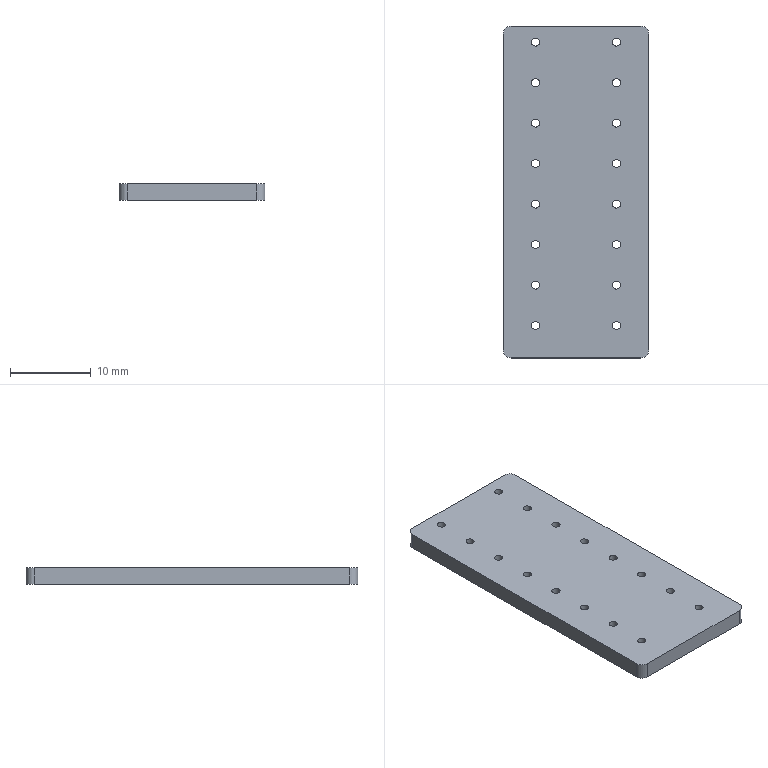Part | NX | features EXTRACT_BODY 7, DATUM_CSYS 3, EXTRUDE 2, SKETCH 2, Pattern Geometry 1, SUBTRACT 1 | 1 solid | 26 faces | box 18 x 41 x 2 mm | volume 1449 mm3 | cylinder 20 | plane 6 | commonest cylinder face diameters 1 x16 2 x4
STEP:
#1=CARTESIAN_POINT('',(-4.5,3.5,0.));
#2=VERTEX_POINT('',#1);
#3=CARTESIAN_POINT('',(-5.,3.5,0.));
#4=DIRECTION('',(0.,0.,1.));
#5=DIRECTION('',(1.,0.,0.));
#6=AXIS2_PLACEMENT_3D('',#3,#4,#5);
#7=CIRCLE('',#6,0.5);
#8=EDGE_CURVE('',#2,#2,#7,.T.);
#9=ORIENTED_EDGE('',*,*,#8,.T.);
#10=EDGE_LOOP('',(#9));
#11=FACE_BOUND('',#10,.T.);
#12=CARTESIAN_POINT('',(-4.5,-1.5,0.));
#13=VERTEX_POINT('',#12);
#14=CARTESIAN_POINT('',(-5.,-1.5,0.));
#15=DIRECTION('',(0.,0.,1.));
#16=DIRECTION('',(1.,0.,0.));
#17=AXIS2_PLACEMENT_3D('',#14,#15,#16);
#18=CIRCLE('',#17,0.5);
#19=EDGE_CURVE('',#13,#13,#18,.T.);
#20=ORIENTED_EDGE('',*,*,#19,.T.);
#21=EDGE_LOOP('',(#20));
#22=FACE_BOUND('',#21,.T.);
#23=CARTESIAN_POINT('',(-4.5,13.5,0.));
#24=VERTEX_POINT('',#23);
#25=CARTESIAN_POINT('',(-5.,13.5,0.));
#26=DIRECTION('',(0.,0.,1.));
#27=DIRECTION('',(1.,0.,0.));
#28=AXIS2_PLACEMENT_3D('',#25,#26,#27);
#29=CIRCLE('',#28,0.5);
#30=EDGE_CURVE('',#24,#24,#29,.T.);
#31=ORIENTED_EDGE('',*,*,#30,.T.);
#32=EDGE_LOOP('',(#31));
#33=FACE_BOUND('',#32,.T.);
#34=CARTESIAN_POINT('',(-4.5,8.5,0.));
#35=VERTEX_POINT('',#34);
#36=CARTESIAN_POINT('',(-5.,8.5,0.));
#37=DIRECTION('',(0.,0.,1.));
#38=DIRECTION('',(1.,0.,0.));
#39=AXIS2_PLACEMENT_3D('',#36,#37,#38);
#40=CIRCLE('',#39,0.5);
#41=EDGE_CURVE('',#35,#35,#40,.T.);
#42=ORIENTED_EDGE('',*,*,#41,.T.);
#43=EDGE_LOOP('',(#42));
#44=FACE_BOUND('',#43,.T.);
#45=CARTESIAN_POINT('',(-4.5,-16.5,0.));
#46=VERTEX_POINT('',#45);
#47=CARTESIAN_POINT('',(-5.,-16.5,0.));
#48=DIRECTION('',(0.,0.,1.));
#49=DIRECTION('',(1.,0.,0.));
#50=AXIS2_PLACEMENT_3D('',#47,#48,#49);
#51=CIRCLE('',#50,0.5);
#52=EDGE_CURVE('',#46,#46,#51,.T.);
#53=ORIENTED_EDGE('',*,*,#52,.T.);
#54=EDGE_LOOP('',(#53));
#55=FACE_BOUND('',#54,.T.);
#56=CARTESIAN_POINT('',(-4.5,-6.5,0.));
#57=VERTEX_POINT('',#56);
#58=CARTESIAN_POINT('',(-5.,-6.5,0.));
#59=DIRECTION('',(0.,0.,1.));
#60=DIRECTION('',(1.,0.,0.));
#61=AXIS2_PLACEMENT_3D('',#58,#59,#60);
#62=CIRCLE('',#61,0.5);
#63=EDGE_CURVE('',#57,#57,#62,.T.);
#64=ORIENTED_EDGE('',*,*,#63,.T.);
#65=EDGE_LOOP('',(#64));
#66=FACE_BOUND('',#65,.T.);
#67=CARTESIAN_POINT('',(-4.5,-11.5,0.));
#68=VERTEX_POINT('',#67);
#69=CARTESIAN_POINT('',(-5.,-11.5,0.));
#70=DIRECTION('',(0.,0.,1.));
#71=DIRECTION('',(1.,0.,0.));
#72=AXIS2_PLACEMENT_3D('',#69,#70,#71);
#73=CIRCLE('',#72,0.5);
#74=EDGE_CURVE('',#68,#68,#73,.T.);
#75=ORIENTED_EDGE('',*,*,#74,.T.);
#76=EDGE_LOOP('',(#75));
#77=FACE_BOUND('',#76,.T.);
#78=CARTESIAN_POINT('',(-4.5,18.5,0.));
#79=VERTEX_POINT('',#78);
#80=CARTESIAN_POINT('',(-5.,18.5,0.));
#81=DIRECTION('',(0.,0.,1.));
#82=DIRECTION('',(1.,0.,0.));
#83=AXIS2_PLACEMENT_3D('',#80,#81,#82);
#84=CIRCLE('',#83,0.5);
#85=EDGE_CURVE('',#79,#79,#84,.T.);
#86=ORIENTED_EDGE('',*,*,#85,.T.);
#87=EDGE_LOOP('',(#86));
#88=FACE_BOUND('',#87,.T.);
#89=CARTESIAN_POINT('',(-9.,19.5,0.));
#90=VERTEX_POINT('',#89);
#91=CARTESIAN_POINT('',(-9.,-19.5,0.));
#92=VERTEX_POINT('',#91);
#93=CARTESIAN_POINT('',(-9.,19.5,0.));
#94=DIRECTION('',(0.,-1.,0.));
#95=VECTOR('',#94,1000.);
#96=LINE('',#93,#95);
#97=EDGE_CURVE('',#90,#92,#96,.T.);
#98=ORIENTED_EDGE('',*,*,#97,.F.);
#99=CARTESIAN_POINT('',(-8.,20.5,0.));
#100=VERTEX_POINT('',#99);
#101=CARTESIAN_POINT('',(-8.,19.5,0.));
#102=DIRECTION('',(0.,0.,1.));
#103=DIRECTION('',(1.,0.,0.));
#104=AXIS2_PLACEMENT_3D('',#101,#102,#103);
#105=CIRCLE('',#104,1.);
#106=EDGE_CURVE('',#100,#90,#105,.T.);
#107=ORIENTED_EDGE('',*,*,#106,.F.);
#108=CARTESIAN_POINT('',(8.,20.5,0.));
#109=VERTEX_POINT('',#108);
#110=CARTESIAN_POINT('',(8.,20.5,0.));
#111=DIRECTION('',(-1.,0.,0.));
#112=VECTOR('',#111,1000.);
#113=LINE('',#110,#112);
#114=EDGE_CURVE('',#109,#100,#113,.T.);
#115=ORIENTED_EDGE('',*,*,#114,.F.);
#116=CARTESIAN_POINT('',(9.,19.5,0.));
#117=VERTEX_POINT('',#116);
#118=CARTESIAN_POINT('',(8.,19.5,0.));
#119=DIRECTION('',(0.,0.,1.));
#120=DIRECTION('',(1.,0.,0.));
#121=AXIS2_PLACEMENT_3D('',#118,#119,#120);
#122=CIRCLE('',#121,1.);
#123=EDGE_CURVE('',#117,#109,#122,.T.);
#124=ORIENTED_EDGE('',*,*,#123,.F.);
#125=CARTESIAN_POINT('',(9.,-19.5,0.));
#126=VERTEX_POINT('',#125);
#127=CARTESIAN_POINT('',(9.,-19.5,0.));
#128=DIRECTION('',(0.,1.,0.));
#129=VECTOR('',#128,1000.);
#130=LINE('',#127,#129);
#131=EDGE_CURVE('',#126,#117,#130,.T.);
#132=ORIENTED_EDGE('',*,*,#131,.F.);
#133=CARTESIAN_POINT('',(8.,-20.5,0.));
#134=VERTEX_POINT('',#133);
#135=CARTESIAN_POINT('',(8.,-19.5,0.));
#136=DIRECTION('',(0.,0.,1.));
#137=DIRECTION('',(1.,0.,0.));
#138=AXIS2_PLACEMENT_3D('',#135,#136,#137);
#139=CIRCLE('',#138,1.);
#140=EDGE_CURVE('',#134,#126,#139,.T.);
#141=ORIENTED_EDGE('',*,*,#140,.F.);
#142=CARTESIAN_POINT('',(-8.,-20.5,0.));
#143=VERTEX_POINT('',#142);
#144=CARTESIAN_POINT('',(-8.,-20.5,0.));
#145=DIRECTION('',(1.,0.,0.));
#146=VECTOR('',#145,1000.);
#147=LINE('',#144,#146);
#148=EDGE_CURVE('',#143,#134,#147,.T.);
#149=ORIENTED_EDGE('',*,*,#148,.F.);
#150=CARTESIAN_POINT('',(-8.,-19.5,0.));
#151=DIRECTION('',(0.,0.,1.));
#152=DIRECTION('',(1.,0.,0.));
#153=AXIS2_PLACEMENT_3D('',#150,#151,#152);
#154=CIRCLE('',#153,1.);
#155=EDGE_CURVE('',#92,#143,#154,.T.);
#156=ORIENTED_EDGE('',*,*,#155,.F.);
#157=EDGE_LOOP('',(#98,#107,#115,#124,#132,#141,#149,#156));
#158=FACE_BOUND('',#157,.T.);
#159=CARTESIAN_POINT('',(5.5,-6.5,0.));
#160=VERTEX_POINT('',#159);
#161=CARTESIAN_POINT('',(5.,-6.5,0.));
#162=DIRECTION('',(0.,0.,1.));
#163=DIRECTION('',(1.,0.,0.));
#164=AXIS2_PLACEMENT_3D('',#161,#162,#163);
#165=CIRCLE('',#164,0.5);
#166=EDGE_CURVE('',#160,#160,#165,.F.);
#167=ORIENTED_EDGE('',*,*,#166,.F.);
#168=EDGE_LOOP('',(#167));
#169=FACE_BOUND('',#168,.T.);
#170=CARTESIAN_POINT('',(5.5,-1.5,0.));
#171=VERTEX_POINT('',#170);
#172=CARTESIAN_POINT('',(5.,-1.5,0.));
#173=DIRECTION('',(0.,0.,1.));
#174=DIRECTION('',(1.,0.,0.));
#175=AXIS2_PLACEMENT_3D('',#172,#173,#174);
#176=CIRCLE('',#175,0.5);
#177=EDGE_CURVE('',#171,#171,#176,.F.);
#178=ORIENTED_EDGE('',*,*,#177,.F.);
#179=EDGE_LOOP('',(#178));
#180=FACE_BOUND('',#179,.T.);
#181=CARTESIAN_POINT('',(5.5,-16.5,0.));
#182=VERTEX_POINT('',#181);
#183=CARTESIAN_POINT('',(5.,-16.5,0.));
#184=DIRECTION('',(0.,0.,1.));
#185=DIRECTION('',(1.,0.,0.));
#186=AXIS2_PLACEMENT_3D('',#183,#184,#185);
#187=CIRCLE('',#186,0.5);
#188=EDGE_CURVE('',#182,#182,#187,.F.);
#189=ORIENTED_EDGE('',*,*,#188,.F.);
#190=EDGE_LOOP('',(#189));
#191=FACE_BOUND('',#190,.T.);
#192=CARTESIAN_POINT('',(5.5,-11.5,0.));
#193=VERTEX_POINT('',#192);
#194=CARTESIAN_POINT('',(5.,-11.5,0.));
#195=DIRECTION('',(0.,0.,1.));
#196=DIRECTION('',(1.,0.,0.));
#197=AXIS2_PLACEMENT_3D('',#194,#195,#196);
#198=CIRCLE('',#197,0.5);
#199=EDGE_CURVE('',#193,#193,#198,.F.);
#200=ORIENTED_EDGE('',*,*,#199,.F.);
#201=EDGE_LOOP('',(#200));
#202=FACE_BOUND('',#201,.T.);
#203=CARTESIAN_POINT('',(5.5,13.5,0.));
#204=VERTEX_POINT('',#203);
#205=CARTESIAN_POINT('',(5.,13.5,0.));
#206=DIRECTION('',(0.,0.,1.));
#207=DIRECTION('',(1.,0.,0.));
#208=AXIS2_PLACEMENT_3D('',#205,#206,#207);
#209=CIRCLE('',#208,0.5);
#210=EDGE_CURVE('',#204,#204,#209,.F.);
#211=ORIENTED_EDGE('',*,*,#210,.F.);
#212=EDGE_LOOP('',(#211));
#213=FACE_BOUND('',#212,.T.);
#214=CARTESIAN_POINT('',(5.5,18.5,0.));
#215=VERTEX_POINT('',#214);
#216=CARTESIAN_POINT('',(5.,18.5,0.));
#217=DIRECTION('',(0.,0.,1.));
#218=DIRECTION('',(1.,0.,0.));
#219=AXIS2_PLACEMENT_3D('',#216,#217,#218);
#220=CIRCLE('',#219,0.5);
#221=EDGE_CURVE('',#215,#215,#220,.F.);
#222=ORIENTED_EDGE('',*,*,#221,.F.);
#223=EDGE_LOOP('',(#222));
#224=FACE_BOUND('',#223,.T.);
#225=CARTESIAN_POINT('',(5.5,3.5,0.));
#226=VERTEX_POINT('',#225);
#227=CARTESIAN_POINT('',(5.,3.5,0.));
#228=DIRECTION('',(0.,0.,1.));
#229=DIRECTION('',(1.,0.,0.));
#230=AXIS2_PLACEMENT_3D('',#227,#228,#229);
#231=CIRCLE('',#230,0.5);
#232=EDGE_CURVE('',#226,#226,#231,.F.);
#233=ORIENTED_EDGE('',*,*,#232,.F.);
#234=EDGE_LOOP('',(#233));
#235=FACE_BOUND('',#234,.T.);
#236=CARTESIAN_POINT('',(5.5,8.5,0.));
#237=VERTEX_POINT('',#236);
#238=CARTESIAN_POINT('',(5.,8.5,0.));
#239=DIRECTION('',(0.,0.,1.));
#240=DIRECTION('',(1.,0.,0.));
#241=AXIS2_PLACEMENT_3D('',#238,#239,#240);
#242=CIRCLE('',#241,0.5);
#243=EDGE_CURVE('',#237,#237,#242,.F.);
#244=ORIENTED_EDGE('',*,*,#243,.F.);
#245=EDGE_LOOP('',(#244));
#246=FACE_BOUND('',#245,.T.);
#247=CARTESIAN_POINT('',(-8.,-19.5,0.));
#248=DIRECTION('',(0.,0.,1.));
#249=DIRECTION('',(1.,0.,0.));
#250=AXIS2_PLACEMENT_3D('',#247,#248,#249);
#251=PLANE('',#250);
#252=ADVANCED_FACE('',(#11,#22,#33,#44,#55,#66,#77,#88,#158,#169,#180,#191,#202,#213,#224,#235,#246),#251,.F.);
#253=CARTESIAN_POINT('',(5.5,3.5,2.));
#254=VERTEX_POINT('',#253);
#255=CARTESIAN_POINT('',(5.,3.5,2.));
#256=DIRECTION('',(0.,0.,1.));
#257=DIRECTION('',(1.,0.,0.));
#258=AXIS2_PLACEMENT_3D('',#255,#256,#257);
#259=CIRCLE('',#258,0.5);
#260=EDGE_CURVE('',#254,#254,#259,.F.);
#261=ORIENTED_EDGE('',*,*,#260,.T.);
#262=EDGE_LOOP('',(#261));
#263=FACE_BOUND('',#262,.T.);
#264=CARTESIAN_POINT('',(-4.5,-1.5,2.));
#265=VERTEX_POINT('',#264);
#266=CARTESIAN_POINT('',(-5.,-1.5,2.));
#267=DIRECTION('',(0.,0.,1.));
#268=DIRECTION('',(1.,0.,0.));
#269=AXIS2_PLACEMENT_3D('',#266,#267,#268);
#270=CIRCLE('',#269,0.5);
#271=EDGE_CURVE('',#265,#265,#270,.T.);
#272=ORIENTED_EDGE('',*,*,#271,.F.);
#273=EDGE_LOOP('',(#272));
#274=FACE_BOUND('',#273,.T.);
#275=CARTESIAN_POINT('',(5.5,13.5,2.));
#276=VERTEX_POINT('',#275);
#277=CARTESIAN_POINT('',(5.,13.5,2.));
#278=DIRECTION('',(0.,0.,1.));
#279=DIRECTION('',(1.,0.,0.));
#280=AXIS2_PLACEMENT_3D('',#277,#278,#279);
#281=CIRCLE('',#280,0.5);
#282=EDGE_CURVE('',#276,#276,#281,.F.);
#283=ORIENTED_EDGE('',*,*,#282,.T.);
#284=EDGE_LOOP('',(#283));
#285=FACE_BOUND('',#284,.T.);
#286=CARTESIAN_POINT('',(-4.5,8.5,2.));
#287=VERTEX_POINT('',#286);
#288=CARTESIAN_POINT('',(-5.,8.5,2.));
#289=DIRECTION('',(0.,0.,1.));
#290=DIRECTION('',(1.,0.,0.));
#291=AXIS2_PLACEMENT_3D('',#288,#289,#290);
#292=CIRCLE('',#291,0.5);
#293=EDGE_CURVE('',#287,#287,#292,.T.);
#294=ORIENTED_EDGE('',*,*,#293,.F.);
#295=EDGE_LOOP('',(#294));
#296=FACE_BOUND('',#295,.T.);
#297=CARTESIAN_POINT('',(5.5,-16.5,2.));
#298=VERTEX_POINT('',#297);
#299=CARTESIAN_POINT('',(5.,-16.5,2.));
#300=DIRECTION('',(0.,0.,1.));
#301=DIRECTION('',(1.,0.,0.));
#302=AXIS2_PLACEMENT_3D('',#299,#300,#301);
#303=CIRCLE('',#302,0.5);
#304=EDGE_CURVE('',#298,#298,#303,.F.);
#305=ORIENTED_EDGE('',*,*,#304,.T.);
#306=EDGE_LOOP('',(#305));
#307=FACE_BOUND('',#306,.T.);
#308=CARTESIAN_POINT('',(5.5,-6.5,2.));
#309=VERTEX_POINT('',#308);
#310=CARTESIAN_POINT('',(5.,-6.5,2.));
#311=DIRECTION('',(0.,0.,1.));
#312=DIRECTION('',(1.,0.,0.));
#313=AXIS2_PLACEMENT_3D('',#310,#311,#312);
#314=CIRCLE('',#313,0.5);
#315=EDGE_CURVE('',#309,#309,#314,.F.);
#316=ORIENTED_EDGE('',*,*,#315,.T.);
#317=EDGE_LOOP('',(#316));
#318=FACE_BOUND('',#317,.T.);
#319=CARTESIAN_POINT('',(-4.5,-11.5,2.));
#320=VERTEX_POINT('',#319);
#321=CARTESIAN_POINT('',(-5.,-11.5,2.));
#322=DIRECTION('',(0.,0.,1.));
#323=DIRECTION('',(1.,0.,0.));
#324=AXIS2_PLACEMENT_3D('',#321,#322,#323);
#325=CIRCLE('',#324,0.5);
#326=EDGE_CURVE('',#320,#320,#325,.T.);
#327=ORIENTED_EDGE('',*,*,#326,.F.);
#328=EDGE_LOOP('',(#327));
#329=FACE_BOUND('',#328,.T.);
#330=CARTESIAN_POINT('',(-4.5,18.5,2.));
#331=VERTEX_POINT('',#330);
#332=CARTESIAN_POINT('',(-5.,18.5,2.));
#333=DIRECTION('',(0.,0.,1.));
#334=DIRECTION('',(1.,0.,0.));
#335=AXIS2_PLACEMENT_3D('',#332,#333,#334);
#336=CIRCLE('',#335,0.5);
#337=EDGE_CURVE('',#331,#331,#336,.T.);
#338=ORIENTED_EDGE('',*,*,#337,.F.);
#339=EDGE_LOOP('',(#338));
#340=FACE_BOUND('',#339,.T.);
#341=CARTESIAN_POINT('',(-9.,19.5,2.));
#342=VERTEX_POINT('',#341);
#343=CARTESIAN_POINT('',(-9.,-19.5,2.));
#344=VERTEX_POINT('',#343);
#345=CARTESIAN_POINT('',(-9.,19.5,2.));
#346=DIRECTION('',(0.,-1.,0.));
#347=VECTOR('',#346,1000.);
#348=LINE('',#345,#347);
#349=EDGE_CURVE('',#342,#344,#348,.T.);
#350=ORIENTED_EDGE('',*,*,#349,.T.);
#351=CARTESIAN_POINT('',(-8.,-20.5,2.));
#352=VERTEX_POINT('',#351);
#353=CARTESIAN_POINT('',(-8.,-19.5,2.));
#354=DIRECTION('',(0.,0.,1.));
#355=DIRECTION('',(1.,0.,0.));
#356=AXIS2_PLACEMENT_3D('',#353,#354,#355);
#357=CIRCLE('',#356,1.);
#358=EDGE_CURVE('',#344,#352,#357,.T.);
#359=ORIENTED_EDGE('',*,*,#358,.T.);
#360=CARTESIAN_POINT('',(8.,-20.5,2.));
#361=VERTEX_POINT('',#360);
#362=CARTESIAN_POINT('',(-8.,-20.5,2.));
#363=DIRECTION('',(1.,0.,0.));
#364=VECTOR('',#363,1000.);
#365=LINE('',#362,#364);
#366=EDGE_CURVE('',#352,#361,#365,.T.);
#367=ORIENTED_EDGE('',*,*,#366,.T.);
#368=CARTESIAN_POINT('',(9.,-19.5,2.));
#369=VERTEX_POINT('',#368);
#370=CARTESIAN_POINT('',(8.,-19.5,2.));
#371=DIRECTION('',(0.,0.,1.));
#372=DIRECTION('',(1.,0.,0.));
#373=AXIS2_PLACEMENT_3D('',#370,#371,#372);
#374=CIRCLE('',#373,1.);
#375=EDGE_CURVE('',#361,#369,#374,.T.);
#376=ORIENTED_EDGE('',*,*,#375,.T.);
#377=CARTESIAN_POINT('',(9.,19.5,2.));
#378=VERTEX_POINT('',#377);
#379=CARTESIAN_POINT('',(9.,-19.5,2.));
#380=DIRECTION('',(0.,1.,0.));
#381=VECTOR('',#380,1000.);
#382=LINE('',#379,#381);
#383=EDGE_CURVE('',#369,#378,#382,.T.);
#384=ORIENTED_EDGE('',*,*,#383,.T.);
#385=CARTESIAN_POINT('',(8.,20.5,2.));
#386=VERTEX_POINT('',#385);
#387=CARTESIAN_POINT('',(8.,19.5,2.));
#388=DIRECTION('',(0.,0.,1.));
#389=DIRECTION('',(1.,0.,0.));
#390=AXIS2_PLACEMENT_3D('',#387,#388,#389);
#391=CIRCLE('',#390,1.);
#392=EDGE_CURVE('',#378,#386,#391,.T.);
#393=ORIENTED_EDGE('',*,*,#392,.T.);
#394=CARTESIAN_POINT('',(-8.,20.5,2.));
#395=VERTEX_POINT('',#394);
#396=CARTESIAN_POINT('',(8.,20.5,2.));
#397=DIRECTION('',(-1.,0.,0.));
#398=VECTOR('',#397,1000.);
#399=LINE('',#396,#398);
#400=EDGE_CURVE('',#386,#395,#399,.T.);
#401=ORIENTED_EDGE('',*,*,#400,.T.);
#402=CARTESIAN_POINT('',(-8.,19.5,2.));
#403=DIRECTION('',(0.,0.,1.));
#404=DIRECTION('',(1.,0.,0.));
#405=AXIS2_PLACEMENT_3D('',#402,#403,#404);
#406=CIRCLE('',#405,1.);
#407=EDGE_CURVE('',#395,#342,#406,.T.);
#408=ORIENTED_EDGE('',*,*,#407,.T.);
#409=EDGE_LOOP('',(#350,#359,#367,#376,#384,#393,#401,#408));
#410=FACE_BOUND('',#409,.T.);
#411=CARTESIAN_POINT('',(-4.5,-6.5,2.));
#412=VERTEX_POINT('',#411);
#413=CARTESIAN_POINT('',(-5.,-6.5,2.));
#414=DIRECTION('',(0.,0.,1.));
#415=DIRECTION('',(1.,0.,0.));
#416=AXIS2_PLACEMENT_3D('',#413,#414,#415);
#417=CIRCLE('',#416,0.5);
#418=EDGE_CURVE('',#412,#412,#417,.T.);
#419=ORIENTED_EDGE('',*,*,#418,.F.);
#420=EDGE_LOOP('',(#419));
#421=FACE_BOUND('',#420,.T.);
#422=CARTESIAN_POINT('',(5.5,-1.5,2.));
#423=VERTEX_POINT('',#422);
#424=CARTESIAN_POINT('',(5.,-1.5,2.));
#425=DIRECTION('',(0.,0.,1.));
#426=DIRECTION('',(1.,0.,0.));
#427=AXIS2_PLACEMENT_3D('',#424,#425,#426);
#428=CIRCLE('',#427,0.5);
#429=EDGE_CURVE('',#423,#423,#428,.F.);
#430=ORIENTED_EDGE('',*,*,#429,.T.);
#431=EDGE_LOOP('',(#430));
#432=FACE_BOUND('',#431,.T.);
#433=CARTESIAN_POINT('',(-4.5,-16.5,2.));
#434=VERTEX_POINT('',#433);
#435=CARTESIAN_POINT('',(-5.,-16.5,2.));
#436=DIRECTION('',(0.,0.,1.));
#437=DIRECTION('',(1.,0.,0.));
#438=AXIS2_PLACEMENT_3D('',#435,#436,#437);
#439=CIRCLE('',#438,0.5);
#440=EDGE_CURVE('',#434,#434,#439,.T.);
#441=ORIENTED_EDGE('',*,*,#440,.F.);
#442=EDGE_LOOP('',(#441));
#443=FACE_BOUND('',#442,.T.);
#444=CARTESIAN_POINT('',(5.5,-11.5,2.));
#445=VERTEX_POINT('',#444);
#446=CARTESIAN_POINT('',(5.,-11.5,2.));
#447=DIRECTION('',(0.,0.,1.));
#448=DIRECTION('',(1.,0.,0.));
#449=AXIS2_PLACEMENT_3D('',#446,#447,#448);
#450=CIRCLE('',#449,0.5);
#451=EDGE_CURVE('',#445,#445,#450,.F.);
#452=ORIENTED_EDGE('',*,*,#451,.T.);
#453=EDGE_LOOP('',(#452));
#454=FACE_BOUND('',#453,.T.);
#455=CARTESIAN_POINT('',(-4.5,13.5,2.));
#456=VERTEX_POINT('',#455);
#457=CARTESIAN_POINT('',(-5.,13.5,2.));
#458=DIRECTION('',(0.,0.,1.));
#459=DIRECTION('',(1.,0.,0.));
#460=AXIS2_PLACEMENT_3D('',#457,#458,#459);
#461=CIRCLE('',#460,0.5);
#462=EDGE_CURVE('',#456,#456,#461,.T.);
#463=ORIENTED_EDGE('',*,*,#462,.F.);
#464=EDGE_LOOP('',(#463));
#465=FACE_BOUND('',#464,.T.);
#466=CARTESIAN_POINT('',(5.5,18.5,2.));
#467=VERTEX_POINT('',#466);
#468=CARTESIAN_POINT('',(5.,18.5,2.));
#469=DIRECTION('',(0.,0.,1.));
#470=DIRECTION('',(1.,0.,0.));
#471=AXIS2_PLACEMENT_3D('',#468,#469,#470);
#472=CIRCLE('',#471,0.5);
#473=EDGE_CURVE('',#467,#467,#472,.F.);
#474=ORIENTED_EDGE('',*,*,#473,.T.);
#475=EDGE_LOOP('',(#474));
#476=FACE_BOUND('',#475,.T.);
#477=CARTESIAN_POINT('',(-4.5,3.5,2.));
#478=VERTEX_POINT('',#477);
#479=CARTESIAN_POINT('',(-5.,3.5,2.));
#480=DIRECTION('',(0.,0.,1.));
#481=DIRECTION('',(1.,0.,0.));
#482=AXIS2_PLACEMENT_3D('',#479,#480,#481);
#483=CIRCLE('',#482,0.5);
#484=EDGE_CURVE('',#478,#478,#483,.T.);
#485=ORIENTED_EDGE('',*,*,#484,.F.);
#486=EDGE_LOOP('',(#485));
#487=FACE_BOUND('',#486,.T.);
#488=CARTESIAN_POINT('',(5.5,8.5,2.));
#489=VERTEX_POINT('',#488);
#490=CARTESIAN_POINT('',(5.,8.5,2.));
#491=DIRECTION('',(0.,0.,1.));
#492=DIRECTION('',(1.,0.,0.));
#493=AXIS2_PLACEMENT_3D('',#490,#491,#492);
#494=CIRCLE('',#493,0.5);
#495=EDGE_CURVE('',#489,#489,#494,.F.);
#496=ORIENTED_EDGE('',*,*,#495,.T.);
#497=EDGE_LOOP('',(#496));
#498=FACE_BOUND('',#497,.T.);
#499=CARTESIAN_POINT('',(-8.,-19.5,2.));
#500=DIRECTION('',(0.,0.,1.));
#501=DIRECTION('',(1.,0.,0.));
#502=AXIS2_PLACEMENT_3D('',#499,#500,#501);
#503=PLANE('',#502);
#504=ADVANCED_FACE('',(#263,#274,#285,#296,#307,#318,#329,#340,#410,#421,#432,#443,#454,#465,#476,#487,#498),#503,.T.);
#505=ORIENTED_EDGE('',*,*,#349,.F.);
#506=CARTESIAN_POINT('',(-9.,19.5,0.));
#507=DIRECTION('',(0.,0.,1.));
#508=VECTOR('',#507,1000.);
#509=LINE('',#506,#508);
#510=EDGE_CURVE('',#90,#342,#509,.T.);
#511=ORIENTED_EDGE('',*,*,#510,.F.);
#512=ORIENTED_EDGE('',*,*,#97,.T.);
#513=CARTESIAN_POINT('',(-9.,-19.5,0.));
#514=DIRECTION('',(0.,0.,1.));
#515=VECTOR('',#514,1000.);
#516=LINE('',#513,#515);
#517=EDGE_CURVE('',#92,#344,#516,.T.);
#518=ORIENTED_EDGE('',*,*,#517,.T.);
#519=EDGE_LOOP('',(#505,#511,#512,#518));
#520=FACE_BOUND('',#519,.T.);
#521=CARTESIAN_POINT('',(-9.,19.5,0.));
#522=DIRECTION('',(-1.,0.,0.));
#523=DIRECTION('',(0.,-1.,0.));
#524=AXIS2_PLACEMENT_3D('',#521,#522,#523);
#525=PLANE('',#524);
#526=ADVANCED_FACE('',(#520),#525,.T.);
#527=ORIENTED_EDGE('',*,*,#358,.F.);
#528=ORIENTED_EDGE('',*,*,#517,.F.);
#529=ORIENTED_EDGE('',*,*,#155,.T.);
#530=CARTESIAN_POINT('',(-8.,-20.5,0.));
#531=DIRECTION('',(0.,0.,1.));
#532=VECTOR('',#531,1000.);
#533=LINE('',#530,#532);
#534=EDGE_CURVE('',#143,#352,#533,.T.);
#535=ORIENTED_EDGE('',*,*,#534,.T.);
#536=EDGE_LOOP('',(#527,#528,#529,#535));
#537=FACE_BOUND('',#536,.T.);
#538=CARTESIAN_POINT('',(-8.,-19.5,0.));
#539=DIRECTION('',(0.,0.,1.));
#540=DIRECTION('',(1.,0.,0.));
#541=AXIS2_PLACEMENT_3D('',#538,#539,#540);
#542=CYLINDRICAL_SURFACE('',#541,1.);
#543=ADVANCED_FACE('',(#537),#542,.T.);
#544=ORIENTED_EDGE('',*,*,#366,.F.);
#545=ORIENTED_EDGE('',*,*,#534,.F.);
#546=ORIENTED_EDGE('',*,*,#148,.T.);
#547=CARTESIAN_POINT('',(8.,-20.5,0.));
#548=DIRECTION('',(0.,0.,1.));
#549=VECTOR('',#548,1000.);
#550=LINE('',#547,#549);
#551=EDGE_CURVE('',#134,#361,#550,.T.);
#552=ORIENTED_EDGE('',*,*,#551,.T.);
#553=EDGE_LOOP('',(#544,#545,#546,#552));
#554=FACE_BOUND('',#553,.T.);
#555=CARTESIAN_POINT('',(-8.,-20.5,0.));
#556=DIRECTION('',(0.,-1.,0.));
#557=DIRECTION('',(0.,0.,-1.));
#558=AXIS2_PLACEMENT_3D('',#555,#556,#557);
#559=PLANE('',#558);
#560=ADVANCED_FACE('',(#554),#559,.T.);
#561=ORIENTED_EDGE('',*,*,#375,.F.);
#562=ORIENTED_EDGE('',*,*,#551,.F.);
#563=ORIENTED_EDGE('',*,*,#140,.T.);
#564=CARTESIAN_POINT('',(9.,-19.5,0.));
#565=DIRECTION('',(0.,0.,1.));
#566=VECTOR('',#565,1000.);
#567=LINE('',#564,#566);
#568=EDGE_CURVE('',#126,#369,#567,.T.);
#569=ORIENTED_EDGE('',*,*,#568,.T.);
#570=EDGE_LOOP('',(#561,#562,#563,#569));
#571=FACE_BOUND('',#570,.T.);
#572=CARTESIAN_POINT('',(8.,-19.5,0.));
#573=DIRECTION('',(0.,0.,1.));
#574=DIRECTION('',(1.,0.,0.));
#575=AXIS2_PLACEMENT_3D('',#572,#573,#574);
#576=CYLINDRICAL_SURFACE('',#575,1.);
#577=ADVANCED_FACE('',(#571),#576,.T.);
#578=ORIENTED_EDGE('',*,*,#383,.F.);
#579=ORIENTED_EDGE('',*,*,#568,.F.);
#580=ORIENTED_EDGE('',*,*,#131,.T.);
#581=CARTESIAN_POINT('',(9.,19.5,0.));
#582=DIRECTION('',(0.,0.,1.));
#583=VECTOR('',#582,1000.);
#584=LINE('',#581,#583);
#585=EDGE_CURVE('',#117,#378,#584,.T.);
#586=ORIENTED_EDGE('',*,*,#585,.T.);
#587=EDGE_LOOP('',(#578,#579,#580,#586));
#588=FACE_BOUND('',#587,.T.);
#589=CARTESIAN_POINT('',(9.,-19.5,0.));
#590=DIRECTION('',(1.,0.,0.));
#591=DIRECTION('',(0.,1.,0.));
#592=AXIS2_PLACEMENT_3D('',#589,#590,#591);
#593=PLANE('',#592);
#594=ADVANCED_FACE('',(#588),#593,.T.);
#595=ORIENTED_EDGE('',*,*,#392,.F.);
#596=ORIENTED_EDGE('',*,*,#585,.F.);
#597=ORIENTED_EDGE('',*,*,#123,.T.);
#598=CARTESIAN_POINT('',(8.,20.5,0.));
#599=DIRECTION('',(0.,0.,1.));
#600=VECTOR('',#599,1000.);
#601=LINE('',#598,#600);
#602=EDGE_CURVE('',#109,#386,#601,.T.);
#603=ORIENTED_EDGE('',*,*,#602,.T.);
#604=EDGE_LOOP('',(#595,#596,#597,#603));
#605=FACE_BOUND('',#604,.T.);
#606=CARTESIAN_POINT('',(8.,19.5,0.));
#607=DIRECTION('',(0.,0.,1.));
#608=DIRECTION('',(1.,0.,0.));
#609=AXIS2_PLACEMENT_3D('',#606,#607,#608);
#610=CYLINDRICAL_SURFACE('',#609,1.);
#611=ADVANCED_FACE('',(#605),#610,.T.);
#612=ORIENTED_EDGE('',*,*,#400,.F.);
#613=ORIENTED_EDGE('',*,*,#602,.F.);
#614=ORIENTED_EDGE('',*,*,#114,.T.);
#615=CARTESIAN_POINT('',(-8.,20.5,0.));
#616=DIRECTION('',(0.,0.,1.));
#617=VECTOR('',#616,1000.);
#618=LINE('',#615,#617);
#619=EDGE_CURVE('',#100,#395,#618,.T.);
#620=ORIENTED_EDGE('',*,*,#619,.T.);
#621=EDGE_LOOP('',(#612,#613,#614,#620));
#622=FACE_BOUND('',#621,.T.);
#623=CARTESIAN_POINT('',(8.,20.5,0.));
#624=DIRECTION('',(0.,1.,0.));
#625=DIRECTION('',(0.,0.,1.));
#626=AXIS2_PLACEMENT_3D('',#623,#624,#625);
#627=PLANE('',#626);
#628=ADVANCED_FACE('',(#622),#627,.T.);
#629=ORIENTED_EDGE('',*,*,#407,.F.);
#630=ORIENTED_EDGE('',*,*,#619,.F.);
#631=ORIENTED_EDGE('',*,*,#106,.T.);
#632=ORIENTED_EDGE('',*,*,#510,.T.);
#633=EDGE_LOOP('',(#629,#630,#631,#632));
#634=FACE_BOUND('',#633,.T.);
#635=CARTESIAN_POINT('',(-8.,19.5,0.));
#636=DIRECTION('',(0.,0.,1.));
#637=DIRECTION('',(1.,0.,0.));
#638=AXIS2_PLACEMENT_3D('',#635,#636,#637);
#639=CYLINDRICAL_SURFACE('',#638,1.);
#640=ADVANCED_FACE('',(#634),#639,.T.);
#641=ORIENTED_EDGE('',*,*,#337,.T.);
#642=EDGE_LOOP('',(#641));
#643=FACE_BOUND('',#642,.T.);
#644=ORIENTED_EDGE('',*,*,#85,.F.);
#645=EDGE_LOOP('',(#644));
#646=FACE_BOUND('',#645,.T.);
#647=CARTESIAN_POINT('',(-5.,18.5,-2.5));
#648=DIRECTION('',(0.,0.,1.));
#649=DIRECTION('',(1.,0.,0.));
#650=AXIS2_PLACEMENT_3D('',#647,#648,#649);
#651=CYLINDRICAL_SURFACE('',#650,0.5);
#652=ADVANCED_FACE('',(#643,#646),#651,.F.);
#653=ORIENTED_EDGE('',*,*,#326,.T.);
#654=EDGE_LOOP('',(#653));
#655=FACE_BOUND('',#654,.T.);
#656=ORIENTED_EDGE('',*,*,#74,.F.);
#657=EDGE_LOOP('',(#656));
#658=FACE_BOUND('',#657,.T.);
#659=CARTESIAN_POINT('',(-5.,-11.5,-2.5));
#660=DIRECTION('',(0.,0.,1.));
#661=DIRECTION('',(1.,0.,0.));
#662=AXIS2_PLACEMENT_3D('',#659,#660,#661);
#663=CYLINDRICAL_SURFACE('',#662,0.5);
#664=ADVANCED_FACE('',(#655,#658),#663,.F.);
#665=ORIENTED_EDGE('',*,*,#315,.F.);
#666=EDGE_LOOP('',(#665));
#667=FACE_BOUND('',#666,.T.);
#668=ORIENTED_EDGE('',*,*,#166,.T.);
#669=EDGE_LOOP('',(#668));
#670=FACE_BOUND('',#669,.T.);
#671=CARTESIAN_POINT('',(5.,-6.5,-2.5));
#672=DIRECTION('',(0.,0.,1.));
#673=DIRECTION('',(1.,0.,0.));
#674=AXIS2_PLACEMENT_3D('',#671,#672,#673);
#675=CYLINDRICAL_SURFACE('',#674,0.5);
#676=ADVANCED_FACE('',(#667,#670),#675,.F.);
#677=ORIENTED_EDGE('',*,*,#418,.T.);
#678=EDGE_LOOP('',(#677));
#679=FACE_BOUND('',#678,.T.);
#680=ORIENTED_EDGE('',*,*,#63,.F.);
#681=EDGE_LOOP('',(#680));
#682=FACE_BOUND('',#681,.T.);
#683=CARTESIAN_POINT('',(-5.,-6.5,-2.5));
#684=DIRECTION('',(0.,0.,1.));
#685=DIRECTION('',(1.,0.,0.));
#686=AXIS2_PLACEMENT_3D('',#683,#684,#685);
#687=CYLINDRICAL_SURFACE('',#686,0.5);
#688=ADVANCED_FACE('',(#679,#682),#687,.F.);
#689=ORIENTED_EDGE('',*,*,#429,.F.);
#690=EDGE_LOOP('',(#689));
#691=FACE_BOUND('',#690,.T.);
#692=ORIENTED_EDGE('',*,*,#177,.T.);
#693=EDGE_LOOP('',(#692));
#694=FACE_BOUND('',#693,.T.);
#695=CARTESIAN_POINT('',(5.,-1.5,-2.5));
#696=DIRECTION('',(0.,0.,1.));
#697=DIRECTION('',(1.,0.,0.));
#698=AXIS2_PLACEMENT_3D('',#695,#696,#697);
#699=CYLINDRICAL_SURFACE('',#698,0.5);
#700=ADVANCED_FACE('',(#691,#694),#699,.F.);
#701=ORIENTED_EDGE('',*,*,#304,.F.);
#702=EDGE_LOOP('',(#701));
#703=FACE_BOUND('',#702,.T.);
#704=ORIENTED_EDGE('',*,*,#188,.T.);
#705=EDGE_LOOP('',(#704));
#706=FACE_BOUND('',#705,.T.);
#707=CARTESIAN_POINT('',(5.,-16.5,-2.5));
#708=DIRECTION('',(0.,0.,1.));
#709=DIRECTION('',(1.,0.,0.));
#710=AXIS2_PLACEMENT_3D('',#707,#708,#709);
#711=CYLINDRICAL_SURFACE('',#710,0.5);
#712=ADVANCED_FACE('',(#703,#706),#711,.F.);
#713=ORIENTED_EDGE('',*,*,#440,.T.);
#714=EDGE_LOOP('',(#713));
#715=FACE_BOUND('',#714,.T.);
#716=ORIENTED_EDGE('',*,*,#52,.F.);
#717=EDGE_LOOP('',(#716));
#718=FACE_BOUND('',#717,.T.);
#719=CARTESIAN_POINT('',(-5.,-16.5,-2.5));
#720=DIRECTION('',(0.,0.,1.));
#721=DIRECTION('',(1.,0.,0.));
#722=AXIS2_PLACEMENT_3D('',#719,#720,#721);
#723=CYLINDRICAL_SURFACE('',#722,0.5);
#724=ADVANCED_FACE('',(#715,#718),#723,.F.);
#725=ORIENTED_EDGE('',*,*,#451,.F.);
#726=EDGE_LOOP('',(#725));
#727=FACE_BOUND('',#726,.T.);
#728=ORIENTED_EDGE('',*,*,#199,.T.);
#729=EDGE_LOOP('',(#728));
#730=FACE_BOUND('',#729,.T.);
#731=CARTESIAN_POINT('',(5.,-11.5,-2.5));
#732=DIRECTION('',(0.,0.,1.));
#733=DIRECTION('',(1.,0.,0.));
#734=AXIS2_PLACEMENT_3D('',#731,#732,#733);
#735=CYLINDRICAL_SURFACE('',#734,0.5);
#736=ADVANCED_FACE('',(#727,#730),#735,.F.);
#737=ORIENTED_EDGE('',*,*,#293,.T.);
#738=EDGE_LOOP('',(#737));
#739=FACE_BOUND('',#738,.T.);
#740=ORIENTED_EDGE('',*,*,#41,.F.);
#741=EDGE_LOOP('',(#740));
#742=FACE_BOUND('',#741,.T.);
#743=CARTESIAN_POINT('',(-5.,8.5,-2.5));
#744=DIRECTION('',(0.,0.,1.));
#745=DIRECTION('',(1.,0.,0.));
#746=AXIS2_PLACEMENT_3D('',#743,#744,#745);
#747=CYLINDRICAL_SURFACE('',#746,0.5);
#748=ADVANCED_FACE('',(#739,#742),#747,.F.);
#749=ORIENTED_EDGE('',*,*,#282,.F.);
#750=EDGE_LOOP('',(#749));
#751=FACE_BOUND('',#750,.T.);
#752=ORIENTED_EDGE('',*,*,#210,.T.);
#753=EDGE_LOOP('',(#752));
#754=FACE_BOUND('',#753,.T.);
#755=CARTESIAN_POINT('',(5.,13.5,-2.5));
#756=DIRECTION('',(0.,0.,1.));
#757=DIRECTION('',(1.,0.,0.));
#758=AXIS2_PLACEMENT_3D('',#755,#756,#757);
#759=CYLINDRICAL_SURFACE('',#758,0.5);
#760=ADVANCED_FACE('',(#751,#754),#759,.F.);
#761=ORIENTED_EDGE('',*,*,#462,.T.);
#762=EDGE_LOOP('',(#761));
#763=FACE_BOUND('',#762,.T.);
#764=ORIENTED_EDGE('',*,*,#30,.F.);
#765=EDGE_LOOP('',(#764));
#766=FACE_BOUND('',#765,.T.);
#767=CARTESIAN_POINT('',(-5.,13.5,-2.5));
#768=DIRECTION('',(0.,0.,1.));
#769=DIRECTION('',(1.,0.,0.));
#770=AXIS2_PLACEMENT_3D('',#767,#768,#769);
#771=CYLINDRICAL_SURFACE('',#770,0.5);
#772=ADVANCED_FACE('',(#763,#766),#771,.F.);
#773=ORIENTED_EDGE('',*,*,#473,.F.);
#774=EDGE_LOOP('',(#773));
#775=FACE_BOUND('',#774,.T.);
#776=ORIENTED_EDGE('',*,*,#221,.T.);
#777=EDGE_LOOP('',(#776));
#778=FACE_BOUND('',#777,.T.);
#779=CARTESIAN_POINT('',(5.,18.5,-2.5));
#780=DIRECTION('',(0.,0.,1.));
#781=DIRECTION('',(1.,0.,0.));
#782=AXIS2_PLACEMENT_3D('',#779,#780,#781);
#783=CYLINDRICAL_SURFACE('',#782,0.5);
#784=ADVANCED_FACE('',(#775,#778),#783,.F.);
#785=ORIENTED_EDGE('',*,*,#271,.T.);
#786=EDGE_LOOP('',(#785));
#787=FACE_BOUND('',#786,.T.);
#788=ORIENTED_EDGE('',*,*,#19,.F.);
#789=EDGE_LOOP('',(#788));
#790=FACE_BOUND('',#789,.T.);
#791=CARTESIAN_POINT('',(-5.,-1.5,-2.5));
#792=DIRECTION('',(0.,0.,1.));
#793=DIRECTION('',(1.,0.,0.));
#794=AXIS2_PLACEMENT_3D('',#791,#792,#793);
#795=CYLINDRICAL_SURFACE('',#794,0.5);
#796=ADVANCED_FACE('',(#787,#790),#795,.F.);
#797=ORIENTED_EDGE('',*,*,#260,.F.);
#798=EDGE_LOOP('',(#797));
#799=FACE_BOUND('',#798,.T.);
#800=ORIENTED_EDGE('',*,*,#232,.T.);
#801=EDGE_LOOP('',(#800));
#802=FACE_BOUND('',#801,.T.);
#803=CARTESIAN_POINT('',(5.,3.5,-2.5));
#804=DIRECTION('',(0.,0.,1.));
#805=DIRECTION('',(1.,0.,0.));
#806=AXIS2_PLACEMENT_3D('',#803,#804,#805);
#807=CYLINDRICAL_SURFACE('',#806,0.5);
#808=ADVANCED_FACE('',(#799,#802),#807,.F.);
#809=ORIENTED_EDGE('',*,*,#484,.T.);
#810=EDGE_LOOP('',(#809));
#811=FACE_BOUND('',#810,.T.);
#812=ORIENTED_EDGE('',*,*,#8,.F.);
#813=EDGE_LOOP('',(#812));
#814=FACE_BOUND('',#813,.T.);
#815=CARTESIAN_POINT('',(-5.,3.5,-2.5));
#816=DIRECTION('',(0.,0.,1.));
#817=DIRECTION('',(1.,0.,0.));
#818=AXIS2_PLACEMENT_3D('',#815,#816,#817);
#819=CYLINDRICAL_SURFACE('',#818,0.5);
#820=ADVANCED_FACE('',(#811,#814),#819,.F.);
#821=ORIENTED_EDGE('',*,*,#495,.F.);
#822=EDGE_LOOP('',(#821));
#823=FACE_BOUND('',#822,.T.);
#824=ORIENTED_EDGE('',*,*,#243,.T.);
#825=EDGE_LOOP('',(#824));
#826=FACE_BOUND('',#825,.T.);
#827=CARTESIAN_POINT('',(5.,8.5,-2.5));
#828=DIRECTION('',(0.,0.,1.));
#829=DIRECTION('',(1.,0.,0.));
#830=AXIS2_PLACEMENT_3D('',#827,#828,#829);
#831=CYLINDRICAL_SURFACE('',#830,0.5);
#832=ADVANCED_FACE('',(#823,#826),#831,.F.);
#833=CLOSED_SHELL('',(#252,#504,#526,#543,#560,#577,#594,#611,#628,#640,#652,#664,#676,#688,#700,#712,#724,#736,#748,#760,#772,#784,#796,#808,#820,#832));
#834=MANIFOLD_SOLID_BREP('',#833);
#835=(LENGTH_UNIT()NAMED_UNIT(*)SI_UNIT(.MILLI.,.METRE.));
#836=UNCERTAINTY_MEASURE_WITH_UNIT(LENGTH_MEASURE(0.00001),#835,'','');
#837=(NAMED_UNIT(*)PLANE_ANGLE_UNIT()SI_UNIT($,.RADIAN.));
#838=(NAMED_UNIT(*)SI_UNIT($,.STERADIAN.)SOLID_ANGLE_UNIT());
#839=(GEOMETRIC_REPRESENTATION_CONTEXT(3)GLOBAL_UNCERTAINTY_ASSIGNED_CONTEXT((#836))GLOBAL_UNIT_ASSIGNED_CONTEXT((#835,#837,#838))REPRESENTATION_CONTEXT('',''));
#840=ADVANCED_BREP_SHAPE_REPRESENTATION('',(#834),#839);